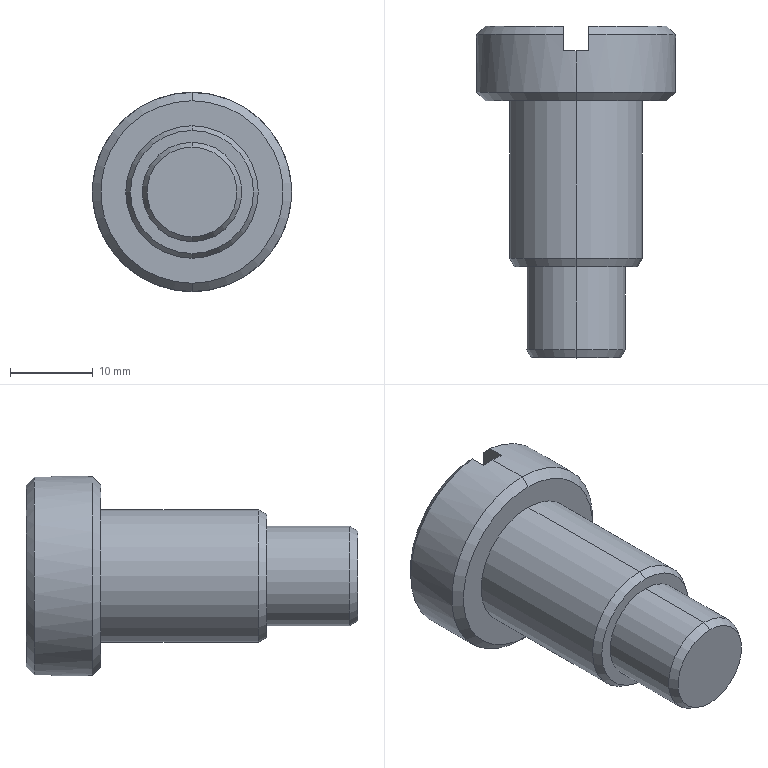Part | SolidWorks | features Chamfer 2, ICE 1, Revolution 1 | 1 solid | 22 faces | box 24 x 40 x 24 mm | volume 9026 mm3 | cone 8 | plane 8 | cylinder 6 | commonest cylinder face diameters 12 x2 16 x2 24 x2
STEP:
#1=CARTESIAN_POINT('',(0.,0.,-5.423));
#2=VERTEX_POINT('',#1);
#3=CARTESIAN_POINT('',(0.,0.,5.423));
#4=VERTEX_POINT('',#3);
#5=CARTESIAN_POINT('',(0.,0.,0.));
#6=DIRECTION('',(0.,-1.,0.));
#7=DIRECTION('',(0.,0.,-1.));
#8=AXIS2_PLACEMENT_3D('',#5,#6,#7);
#9=CIRCLE('',#8,5.423);
#10=EDGE_CURVE('',#2,#4,#9,.T.);
#11=ORIENTED_EDGE('',*,*,#10,.F.);
#12=CARTESIAN_POINT('',(0.,1.,-6.));
#13=VERTEX_POINT('',#12);
#14=CARTESIAN_POINT('',(0.,0.,-5.423));
#15=DIRECTION('',(0.,0.866,-0.5));
#16=VECTOR('',#15,1000.);
#17=LINE('',#14,#16);
#18=EDGE_CURVE('',#2,#13,#17,.T.);
#19=ORIENTED_EDGE('',*,*,#18,.T.);
#20=CARTESIAN_POINT('',(0.,1.,6.));
#21=VERTEX_POINT('',#20);
#22=CARTESIAN_POINT('',(0.,1.,0.));
#23=DIRECTION('',(0.,1.,0.));
#24=DIRECTION('',(0.,0.,-1.));
#25=AXIS2_PLACEMENT_3D('',#22,#23,#24);
#26=CIRCLE('',#25,6.);
#27=EDGE_CURVE('',#21,#13,#26,.T.);
#28=ORIENTED_EDGE('',*,*,#27,.F.);
#29=CARTESIAN_POINT('',(0.,0.,5.423));
#30=DIRECTION('',(0.,0.866,0.5));
#31=VECTOR('',#30,1000.);
#32=LINE('',#29,#31);
#33=EDGE_CURVE('',#4,#21,#32,.T.);
#34=ORIENTED_EDGE('',*,*,#33,.F.);
#35=EDGE_LOOP('',(#11,#19,#28,#34));
#36=FACE_OUTER_BOUND('',#35,.T.);
#37=CARTESIAN_POINT('',(0.,0.,0.));
#38=DIRECTION('',(0.,1.,0.));
#39=DIRECTION('',(0.,0.,1.));
#40=AXIS2_PLACEMENT_3D('',#37,#38,#39);
#41=CONICAL_SURFACE('',#40,5.423,0.5236);
#42=ADVANCED_FACE('',(#36),#41,.T.);
#43=CARTESIAN_POINT('',(0.,11.,-7.423));
#44=VERTEX_POINT('',#43);
#45=CARTESIAN_POINT('',(0.,11.,7.423));
#46=VERTEX_POINT('',#45);
#47=CARTESIAN_POINT('',(0.,11.,0.));
#48=DIRECTION('',(0.,-1.,0.));
#49=DIRECTION('',(0.,0.,-1.));
#50=AXIS2_PLACEMENT_3D('',#47,#48,#49);
#51=CIRCLE('',#50,7.423);
#52=EDGE_CURVE('',#44,#46,#51,.T.);
#53=ORIENTED_EDGE('',*,*,#52,.F.);
#54=CARTESIAN_POINT('',(0.,12.,-8.));
#55=VERTEX_POINT('',#54);
#56=CARTESIAN_POINT('',(0.,11.,-7.423));
#57=DIRECTION('',(0.,0.866,-0.5));
#58=VECTOR('',#57,1000.);
#59=LINE('',#56,#58);
#60=EDGE_CURVE('',#44,#55,#59,.T.);
#61=ORIENTED_EDGE('',*,*,#60,.T.);
#62=CARTESIAN_POINT('',(0.,12.,8.));
#63=VERTEX_POINT('',#62);
#64=CARTESIAN_POINT('',(0.,12.,0.));
#65=DIRECTION('',(0.,1.,0.));
#66=DIRECTION('',(0.,0.,-1.));
#67=AXIS2_PLACEMENT_3D('',#64,#65,#66);
#68=CIRCLE('',#67,8.);
#69=EDGE_CURVE('',#63,#55,#68,.T.);
#70=ORIENTED_EDGE('',*,*,#69,.F.);
#71=CARTESIAN_POINT('',(0.,11.,7.423));
#72=DIRECTION('',(0.,0.866,0.5));
#73=VECTOR('',#72,1000.);
#74=LINE('',#71,#73);
#75=EDGE_CURVE('',#46,#63,#74,.T.);
#76=ORIENTED_EDGE('',*,*,#75,.F.);
#77=EDGE_LOOP('',(#53,#61,#70,#76));
#78=FACE_OUTER_BOUND('',#77,.T.);
#79=CARTESIAN_POINT('',(0.,11.,0.));
#80=DIRECTION('',(0.,1.,0.));
#81=DIRECTION('',(0.,0.,1.));
#82=AXIS2_PLACEMENT_3D('',#79,#80,#81);
#83=CONICAL_SURFACE('',#82,7.423,0.5236);
#84=ADVANCED_FACE('',(#78),#83,.T.);
#85=CARTESIAN_POINT('',(0.,31.,-11.));
#86=VERTEX_POINT('',#85);
#87=CARTESIAN_POINT('',(0.,31.,11.));
#88=VERTEX_POINT('',#87);
#89=CARTESIAN_POINT('',(0.,31.,0.));
#90=DIRECTION('',(0.,-1.,0.));
#91=DIRECTION('',(0.,0.,-1.));
#92=AXIS2_PLACEMENT_3D('',#89,#90,#91);
#93=CIRCLE('',#92,11.);
#94=EDGE_CURVE('',#86,#88,#93,.T.);
#95=ORIENTED_EDGE('',*,*,#94,.F.);
#96=CARTESIAN_POINT('',(0.,32.,-12.));
#97=VERTEX_POINT('',#96);
#98=CARTESIAN_POINT('',(0.,31.,-11.));
#99=DIRECTION('',(0.,0.7071,-0.7071));
#100=VECTOR('',#99,1000.);
#101=LINE('',#98,#100);
#102=EDGE_CURVE('',#86,#97,#101,.T.);
#103=ORIENTED_EDGE('',*,*,#102,.T.);
#104=CARTESIAN_POINT('',(0.,32.,12.));
#105=VERTEX_POINT('',#104);
#106=CARTESIAN_POINT('',(0.,32.,0.));
#107=DIRECTION('',(0.,1.,0.));
#108=DIRECTION('',(0.,0.,-1.));
#109=AXIS2_PLACEMENT_3D('',#106,#107,#108);
#110=CIRCLE('',#109,12.);
#111=EDGE_CURVE('',#105,#97,#110,.T.);
#112=ORIENTED_EDGE('',*,*,#111,.F.);
#113=CARTESIAN_POINT('',(0.,31.,11.));
#114=DIRECTION('',(0.,0.7071,0.7071));
#115=VECTOR('',#114,1000.);
#116=LINE('',#113,#115);
#117=EDGE_CURVE('',#88,#105,#116,.T.);
#118=ORIENTED_EDGE('',*,*,#117,.F.);
#119=EDGE_LOOP('',(#95,#103,#112,#118));
#120=FACE_OUTER_BOUND('',#119,.T.);
#121=CARTESIAN_POINT('',(0.,31.,0.));
#122=DIRECTION('',(0.,1.,0.));
#123=DIRECTION('',(0.,0.,1.));
#124=AXIS2_PLACEMENT_3D('',#121,#122,#123);
#125=CONICAL_SURFACE('',#124,11.,0.7854);
#126=ADVANCED_FACE('',(#120),#125,.T.);
#127=CARTESIAN_POINT('',(0.,11.,-6.));
#128=VERTEX_POINT('',#127);
#129=CARTESIAN_POINT('',(0.,11.,6.));
#130=VERTEX_POINT('',#129);
#131=CARTESIAN_POINT('',(0.,11.,0.));
#132=DIRECTION('',(0.,-1.,0.));
#133=DIRECTION('',(0.,0.,-1.));
#134=AXIS2_PLACEMENT_3D('',#131,#132,#133);
#135=CIRCLE('',#134,6.);
#136=EDGE_CURVE('',#128,#130,#135,.T.);
#137=ORIENTED_EDGE('',*,*,#136,.T.);
#138=CARTESIAN_POINT('',(0.,0.,6.));
#139=DIRECTION('',(0.,-1.,0.));
#140=VECTOR('',#139,1000.);
#141=LINE('',#138,#140);
#142=EDGE_CURVE('',#130,#21,#141,.T.);
#143=ORIENTED_EDGE('',*,*,#142,.T.);
#144=ORIENTED_EDGE('',*,*,#27,.T.);
#145=CARTESIAN_POINT('',(0.,0.,-6.));
#146=DIRECTION('',(0.,-1.,0.));
#147=VECTOR('',#146,1000.);
#148=LINE('',#145,#147);
#149=EDGE_CURVE('',#128,#13,#148,.T.);
#150=ORIENTED_EDGE('',*,*,#149,.F.);
#151=EDGE_LOOP('',(#137,#143,#144,#150));
#152=FACE_OUTER_BOUND('',#151,.T.);
#153=CARTESIAN_POINT('',(0.,0.,0.));
#154=DIRECTION('',(0.,-1.,0.));
#155=DIRECTION('',(0.,0.,-1.));
#156=AXIS2_PLACEMENT_3D('',#153,#154,#155);
#157=CYLINDRICAL_SURFACE('',#156,6.);
#158=ADVANCED_FACE('',(#152),#157,.T.);
#159=CARTESIAN_POINT('',(0.,31.,-8.));
#160=VERTEX_POINT('',#159);
#161=CARTESIAN_POINT('',(0.,31.,8.));
#162=VERTEX_POINT('',#161);
#163=CARTESIAN_POINT('',(0.,31.,0.));
#164=DIRECTION('',(0.,-1.,0.));
#165=DIRECTION('',(0.,0.,-1.));
#166=AXIS2_PLACEMENT_3D('',#163,#164,#165);
#167=CIRCLE('',#166,8.);
#168=EDGE_CURVE('',#160,#162,#167,.T.);
#169=ORIENTED_EDGE('',*,*,#168,.T.);
#170=CARTESIAN_POINT('',(0.,0.,8.));
#171=DIRECTION('',(0.,-1.,0.));
#172=VECTOR('',#171,1000.);
#173=LINE('',#170,#172);
#174=EDGE_CURVE('',#162,#63,#173,.T.);
#175=ORIENTED_EDGE('',*,*,#174,.T.);
#176=ORIENTED_EDGE('',*,*,#69,.T.);
#177=CARTESIAN_POINT('',(0.,0.,-8.));
#178=DIRECTION('',(0.,-1.,0.));
#179=VECTOR('',#178,1000.);
#180=LINE('',#177,#179);
#181=EDGE_CURVE('',#160,#55,#180,.T.);
#182=ORIENTED_EDGE('',*,*,#181,.F.);
#183=EDGE_LOOP('',(#169,#175,#176,#182));
#184=FACE_OUTER_BOUND('',#183,.T.);
#185=CARTESIAN_POINT('',(0.,0.,0.));
#186=DIRECTION('',(0.,-1.,0.));
#187=DIRECTION('',(0.,0.,-1.));
#188=AXIS2_PLACEMENT_3D('',#185,#186,#187);
#189=CYLINDRICAL_SURFACE('',#188,8.);
#190=ADVANCED_FACE('',(#184),#189,.T.);
#191=CARTESIAN_POINT('',(0.,37.,12.));
#192=VERTEX_POINT('',#191);
#193=CARTESIAN_POINT('',(1.5,37.,11.906));
#194=VERTEX_POINT('',#193);
#195=CARTESIAN_POINT('',(0.,37.,0.));
#196=DIRECTION('',(0.,1.,0.));
#197=DIRECTION('',(0.,0.,-1.));
#198=AXIS2_PLACEMENT_3D('',#195,#196,#197);
#199=CIRCLE('',#198,12.);
#200=EDGE_CURVE('',#192,#194,#199,.T.);
#201=ORIENTED_EDGE('',*,*,#200,.F.);
#202=CARTESIAN_POINT('',(0.,0.,12.));
#203=DIRECTION('',(0.,-1.,0.));
#204=VECTOR('',#203,1000.);
#205=LINE('',#202,#204);
#206=EDGE_CURVE('',#192,#105,#205,.T.);
#207=ORIENTED_EDGE('',*,*,#206,.T.);
#208=ORIENTED_EDGE('',*,*,#111,.T.);
#209=CARTESIAN_POINT('',(0.,37.,-12.));
#210=VERTEX_POINT('',#209);
#211=CARTESIAN_POINT('',(0.,0.,-12.));
#212=DIRECTION('',(0.,-1.,0.));
#213=VECTOR('',#212,1000.);
#214=LINE('',#211,#213);
#215=EDGE_CURVE('',#210,#97,#214,.T.);
#216=ORIENTED_EDGE('',*,*,#215,.F.);
#217=CARTESIAN_POINT('',(1.5,37.,-11.906));
#218=VERTEX_POINT('',#217);
#219=CARTESIAN_POINT('',(0.,37.,0.));
#220=DIRECTION('',(0.,1.,0.));
#221=DIRECTION('',(0.,0.,-1.));
#222=AXIS2_PLACEMENT_3D('',#219,#220,#221);
#223=CIRCLE('',#222,12.);
#224=EDGE_CURVE('',#218,#210,#223,.T.);
#225=ORIENTED_EDGE('',*,*,#224,.F.);
#226=CARTESIAN_POINT('',(1.5,39.,-11.906));
#227=VERTEX_POINT('',#226);
#228=CARTESIAN_POINT('',(1.5,0.,-11.906));
#229=DIRECTION('',(0.,-1.,0.));
#230=VECTOR('',#229,1000.);
#231=LINE('',#228,#230);
#232=EDGE_CURVE('',#227,#218,#231,.T.);
#233=ORIENTED_EDGE('',*,*,#232,.F.);
#234=CARTESIAN_POINT('',(1.5,39.,11.906));
#235=VERTEX_POINT('',#234);
#236=CARTESIAN_POINT('',(0.,39.,0.));
#237=DIRECTION('',(0.,-1.,0.));
#238=DIRECTION('',(0.,0.,1.));
#239=AXIS2_PLACEMENT_3D('',#236,#237,#238);
#240=CIRCLE('',#239,12.);
#241=EDGE_CURVE('',#227,#235,#240,.T.);
#242=ORIENTED_EDGE('',*,*,#241,.T.);
#243=CARTESIAN_POINT('',(1.5,0.,11.906));
#244=DIRECTION('',(0.,1.,0.));
#245=VECTOR('',#244,1000.);
#246=LINE('',#243,#245);
#247=EDGE_CURVE('',#194,#235,#246,.T.);
#248=ORIENTED_EDGE('',*,*,#247,.F.);
#249=EDGE_LOOP('',(#201,#207,#208,#216,#225,#233,#242,#248));
#250=FACE_OUTER_BOUND('',#249,.T.);
#251=CARTESIAN_POINT('',(0.,0.,0.));
#252=DIRECTION('',(0.,-1.,0.));
#253=DIRECTION('',(0.,0.,-1.));
#254=AXIS2_PLACEMENT_3D('',#251,#252,#253);
#255=CYLINDRICAL_SURFACE('',#254,12.);
#256=ADVANCED_FACE('',(#250),#255,.T.);
#257=CARTESIAN_POINT('',(1.5,40.,10.897));
#258=VERTEX_POINT('',#257);
#259=CARTESIAN_POINT('',(1.5,40.,-10.897));
#260=VERTEX_POINT('',#259);
#261=CARTESIAN_POINT('',(1.5,40.,15.294));
#262=DIRECTION('',(0.,0.,-1.));
#263=VECTOR('',#262,1000.);
#264=LINE('',#261,#263);
#265=EDGE_CURVE('',#258,#260,#264,.T.);
#266=ORIENTED_EDGE('',*,*,#265,.F.);
#267=CARTESIAN_POINT('',(0.,40.,0.));
#268=DIRECTION('',(0.,1.,0.));
#269=DIRECTION('',(0.,0.,1.));
#270=AXIS2_PLACEMENT_3D('',#267,#268,#269);
#271=CIRCLE('',#270,11.);
#272=EDGE_CURVE('',#258,#260,#271,.T.);
#273=ORIENTED_EDGE('',*,*,#272,.T.);
#274=EDGE_LOOP('',(#266,#273));
#275=FACE_OUTER_BOUND('',#274,.T.);
#276=CARTESIAN_POINT('',(0.,40.,0.));
#277=DIRECTION('',(0.,1.,0.));
#278=DIRECTION('',(0.,0.,1.));
#279=AXIS2_PLACEMENT_3D('',#276,#277,#278);
#280=PLANE('',#279);
#281=ADVANCED_FACE('',(#275),#280,.T.);
#282=CARTESIAN_POINT('',(1.5,39.,11.906));
#283=CARTESIAN_POINT('',(1.5,39.333,11.57));
#284=CARTESIAN_POINT('',(1.5,39.667,11.234));
#285=CARTESIAN_POINT('',(1.5,40.,10.897));
#286=B_SPLINE_CURVE_WITH_KNOTS('',3,(#282,#283,#284,#285),.UNSPECIFIED.,.F.,.F.,(4,4),(0.000000994,0.001421),.UNSPECIFIED.);
#287=EDGE_CURVE('',#235,#258,#286,.T.);
#288=ORIENTED_EDGE('',*,*,#287,.F.);
#289=ORIENTED_EDGE('',*,*,#241,.F.);
#290=CARTESIAN_POINT('',(1.5,40.,-10.897));
#291=CARTESIAN_POINT('',(1.5,39.667,-11.234));
#292=CARTESIAN_POINT('',(1.5,39.333,-11.57));
#293=CARTESIAN_POINT('',(1.5,39.,-11.906));
#294=B_SPLINE_CURVE_WITH_KNOTS('',3,(#290,#291,#292,#293),.UNSPECIFIED.,.F.,.F.,(4,4),(0.03055,0.03197),.UNSPECIFIED.);
#295=EDGE_CURVE('',#260,#227,#294,.T.);
#296=ORIENTED_EDGE('',*,*,#295,.F.);
#297=ORIENTED_EDGE('',*,*,#272,.F.);
#298=EDGE_LOOP('',(#288,#289,#296,#297));
#299=FACE_OUTER_BOUND('',#298,.T.);
#300=CARTESIAN_POINT('',(0.,39.,0.));
#301=DIRECTION('',(0.,-1.,0.));
#302=DIRECTION('',(0.,0.,-1.));
#303=AXIS2_PLACEMENT_3D('',#300,#301,#302);
#304=CONICAL_SURFACE('',#303,12.,0.7854);
#305=ADVANCED_FACE('',(#299),#304,.T.);
#306=CARTESIAN_POINT('',(0.,0.,0.));
#307=DIRECTION('',(0.,-1.,0.));
#308=DIRECTION('',(0.,0.,-1.));
#309=AXIS2_PLACEMENT_3D('',#306,#307,#308);
#310=CIRCLE('',#309,5.423);
#311=EDGE_CURVE('',#4,#2,#310,.T.);
#312=ORIENTED_EDGE('',*,*,#311,.T.);
#313=ORIENTED_EDGE('',*,*,#10,.T.);
#314=EDGE_LOOP('',(#312,#313));
#315=FACE_OUTER_BOUND('',#314,.T.);
#316=CARTESIAN_POINT('',(6.,0.,0.));
#317=DIRECTION('',(0.,-1.,0.));
#318=DIRECTION('',(0.,0.,-1.));
#319=AXIS2_PLACEMENT_3D('',#316,#317,#318);
#320=PLANE('',#319);
#321=ADVANCED_FACE('',(#315),#320,.T.);
#322=CARTESIAN_POINT('',(-1.5,40.,-10.897));
#323=VERTEX_POINT('',#322);
#324=CARTESIAN_POINT('',(-1.5,40.,10.897));
#325=VERTEX_POINT('',#324);
#326=CARTESIAN_POINT('',(-1.5,40.,15.294));
#327=DIRECTION('',(0.,0.,1.));
#328=VECTOR('',#327,1000.);
#329=LINE('',#326,#328);
#330=EDGE_CURVE('',#323,#325,#329,.T.);
#331=ORIENTED_EDGE('',*,*,#330,.F.);
#332=CARTESIAN_POINT('',(0.,40.,0.));
#333=DIRECTION('',(0.,1.,0.));
#334=DIRECTION('',(0.,0.,1.));
#335=AXIS2_PLACEMENT_3D('',#332,#333,#334);
#336=CIRCLE('',#335,11.);
#337=EDGE_CURVE('',#323,#325,#336,.T.);
#338=ORIENTED_EDGE('',*,*,#337,.T.);
#339=EDGE_LOOP('',(#331,#338));
#340=FACE_OUTER_BOUND('',#339,.T.);
#341=CARTESIAN_POINT('',(0.,40.,0.));
#342=DIRECTION('',(0.,1.,0.));
#343=DIRECTION('',(0.,0.,1.));
#344=AXIS2_PLACEMENT_3D('',#341,#342,#343);
#345=PLANE('',#344);
#346=ADVANCED_FACE('',(#340),#345,.T.);
#347=ORIENTED_EDGE('',*,*,#206,.F.);
#348=CARTESIAN_POINT('',(-1.5,37.,11.906));
#349=VERTEX_POINT('',#348);
#350=CARTESIAN_POINT('',(0.,37.,0.));
#351=DIRECTION('',(0.,1.,0.));
#352=DIRECTION('',(0.,0.,-1.));
#353=AXIS2_PLACEMENT_3D('',#350,#351,#352);
#354=CIRCLE('',#353,12.);
#355=EDGE_CURVE('',#349,#192,#354,.T.);
#356=ORIENTED_EDGE('',*,*,#355,.F.);
#357=CARTESIAN_POINT('',(-1.5,39.,11.906));
#358=VERTEX_POINT('',#357);
#359=CARTESIAN_POINT('',(-1.5,0.,11.906));
#360=DIRECTION('',(0.,-1.,0.));
#361=VECTOR('',#360,1000.);
#362=LINE('',#359,#361);
#363=EDGE_CURVE('',#358,#349,#362,.T.);
#364=ORIENTED_EDGE('',*,*,#363,.F.);
#365=CARTESIAN_POINT('',(-1.5,39.,-11.906));
#366=VERTEX_POINT('',#365);
#367=CARTESIAN_POINT('',(0.,39.,0.));
#368=DIRECTION('',(0.,-1.,0.));
#369=DIRECTION('',(0.,0.,1.));
#370=AXIS2_PLACEMENT_3D('',#367,#368,#369);
#371=CIRCLE('',#370,12.);
#372=EDGE_CURVE('',#358,#366,#371,.T.);
#373=ORIENTED_EDGE('',*,*,#372,.T.);
#374=CARTESIAN_POINT('',(-1.5,37.,-11.906));
#375=VERTEX_POINT('',#374);
#376=CARTESIAN_POINT('',(-1.5,0.,-11.906));
#377=DIRECTION('',(0.,1.,0.));
#378=VECTOR('',#377,1000.);
#379=LINE('',#376,#378);
#380=EDGE_CURVE('',#375,#366,#379,.T.);
#381=ORIENTED_EDGE('',*,*,#380,.F.);
#382=CARTESIAN_POINT('',(0.,37.,0.));
#383=DIRECTION('',(0.,1.,0.));
#384=DIRECTION('',(0.,0.,-1.));
#385=AXIS2_PLACEMENT_3D('',#382,#383,#384);
#386=CIRCLE('',#385,12.);
#387=EDGE_CURVE('',#210,#375,#386,.T.);
#388=ORIENTED_EDGE('',*,*,#387,.F.);
#389=ORIENTED_EDGE('',*,*,#215,.T.);
#390=CARTESIAN_POINT('',(0.,32.,0.));
#391=DIRECTION('',(0.,1.,0.));
#392=DIRECTION('',(0.,0.,-1.));
#393=AXIS2_PLACEMENT_3D('',#390,#391,#392);
#394=CIRCLE('',#393,12.);
#395=EDGE_CURVE('',#97,#105,#394,.T.);
#396=ORIENTED_EDGE('',*,*,#395,.T.);
#397=EDGE_LOOP('',(#347,#356,#364,#373,#381,#388,#389,#396));
#398=FACE_OUTER_BOUND('',#397,.T.);
#399=CARTESIAN_POINT('',(0.,0.,0.));
#400=DIRECTION('',(0.,-1.,0.));
#401=DIRECTION('',(0.,0.,-1.));
#402=AXIS2_PLACEMENT_3D('',#399,#400,#401);
#403=CYLINDRICAL_SURFACE('',#402,12.);
#404=ADVANCED_FACE('',(#398),#403,.T.);
#405=CARTESIAN_POINT('',(0.,31.,0.));
#406=DIRECTION('',(0.,-1.,0.));
#407=DIRECTION('',(0.,0.,-1.));
#408=AXIS2_PLACEMENT_3D('',#405,#406,#407);
#409=CIRCLE('',#408,11.);
#410=EDGE_CURVE('',#88,#86,#409,.T.);
#411=ORIENTED_EDGE('',*,*,#410,.T.);
#412=ORIENTED_EDGE('',*,*,#94,.T.);
#413=EDGE_LOOP('',(#411,#412));
#414=FACE_OUTER_BOUND('',#413,.T.);
#415=ORIENTED_EDGE('',*,*,#168,.F.);
#416=CARTESIAN_POINT('',(0.,31.,0.));
#417=DIRECTION('',(0.,-1.,0.));
#418=DIRECTION('',(0.,0.,-1.));
#419=AXIS2_PLACEMENT_3D('',#416,#417,#418);
#420=CIRCLE('',#419,8.);
#421=EDGE_CURVE('',#162,#160,#420,.T.);
#422=ORIENTED_EDGE('',*,*,#421,.F.);
#423=EDGE_LOOP('',(#415,#422));
#424=FACE_BOUND('',#423,.T.);
#425=CARTESIAN_POINT('',(12.,31.,0.));
#426=DIRECTION('',(0.,-1.,0.));
#427=DIRECTION('',(0.,0.,-1.));
#428=AXIS2_PLACEMENT_3D('',#425,#426,#427);
#429=PLANE('',#428);
#430=ADVANCED_FACE('',(#414,#424),#429,.T.);
#431=ORIENTED_EDGE('',*,*,#174,.F.);
#432=ORIENTED_EDGE('',*,*,#421,.T.);
#433=ORIENTED_EDGE('',*,*,#181,.T.);
#434=CARTESIAN_POINT('',(0.,12.,0.));
#435=DIRECTION('',(0.,1.,0.));
#436=DIRECTION('',(0.,0.,-1.));
#437=AXIS2_PLACEMENT_3D('',#434,#435,#436);
#438=CIRCLE('',#437,8.);
#439=EDGE_CURVE('',#55,#63,#438,.T.);
#440=ORIENTED_EDGE('',*,*,#439,.T.);
#441=EDGE_LOOP('',(#431,#432,#433,#440));
#442=FACE_OUTER_BOUND('',#441,.T.);
#443=CARTESIAN_POINT('',(0.,0.,0.));
#444=DIRECTION('',(0.,-1.,0.));
#445=DIRECTION('',(0.,0.,-1.));
#446=AXIS2_PLACEMENT_3D('',#443,#444,#445);
#447=CYLINDRICAL_SURFACE('',#446,8.);
#448=ADVANCED_FACE('',(#442),#447,.T.);
#449=CARTESIAN_POINT('',(0.,11.,0.));
#450=DIRECTION('',(0.,-1.,0.));
#451=DIRECTION('',(0.,0.,-1.));
#452=AXIS2_PLACEMENT_3D('',#449,#450,#451);
#453=CIRCLE('',#452,7.423);
#454=EDGE_CURVE('',#46,#44,#453,.T.);
#455=ORIENTED_EDGE('',*,*,#454,.T.);
#456=ORIENTED_EDGE('',*,*,#52,.T.);
#457=EDGE_LOOP('',(#455,#456));
#458=FACE_OUTER_BOUND('',#457,.T.);
#459=ORIENTED_EDGE('',*,*,#136,.F.);
#460=CARTESIAN_POINT('',(0.,11.,0.));
#461=DIRECTION('',(0.,-1.,0.));
#462=DIRECTION('',(0.,0.,-1.));
#463=AXIS2_PLACEMENT_3D('',#460,#461,#462);
#464=CIRCLE('',#463,6.);
#465=EDGE_CURVE('',#130,#128,#464,.T.);
#466=ORIENTED_EDGE('',*,*,#465,.F.);
#467=EDGE_LOOP('',(#459,#466));
#468=FACE_BOUND('',#467,.T.);
#469=CARTESIAN_POINT('',(8.,11.,0.));
#470=DIRECTION('',(0.,-1.,0.));
#471=DIRECTION('',(0.,0.,-1.));
#472=AXIS2_PLACEMENT_3D('',#469,#470,#471);
#473=PLANE('',#472);
#474=ADVANCED_FACE('',(#458,#468),#473,.T.);
#475=ORIENTED_EDGE('',*,*,#142,.F.);
#476=ORIENTED_EDGE('',*,*,#465,.T.);
#477=ORIENTED_EDGE('',*,*,#149,.T.);
#478=CARTESIAN_POINT('',(0.,1.,0.));
#479=DIRECTION('',(0.,1.,0.));
#480=DIRECTION('',(0.,0.,-1.));
#481=AXIS2_PLACEMENT_3D('',#478,#479,#480);
#482=CIRCLE('',#481,6.);
#483=EDGE_CURVE('',#13,#21,#482,.T.);
#484=ORIENTED_EDGE('',*,*,#483,.T.);
#485=EDGE_LOOP('',(#475,#476,#477,#484));
#486=FACE_OUTER_BOUND('',#485,.T.);
#487=CARTESIAN_POINT('',(0.,0.,0.));
#488=DIRECTION('',(0.,-1.,0.));
#489=DIRECTION('',(0.,0.,-1.));
#490=AXIS2_PLACEMENT_3D('',#487,#488,#489);
#491=CYLINDRICAL_SURFACE('',#490,6.);
#492=ADVANCED_FACE('',(#486),#491,.T.);
#493=CARTESIAN_POINT('',(-1.5,39.,-11.906));
#494=CARTESIAN_POINT('',(-1.5,39.333,-11.57));
#495=CARTESIAN_POINT('',(-1.5,39.667,-11.234));
#496=CARTESIAN_POINT('',(-1.5,40.,-10.897));
#497=B_SPLINE_CURVE_WITH_KNOTS('',3,(#493,#494,#495,#496),.UNSPECIFIED.,.F.,.F.,(4,4),(0.000000994,0.001421),.UNSPECIFIED.);
#498=EDGE_CURVE('',#366,#323,#497,.T.);
#499=ORIENTED_EDGE('',*,*,#498,.F.);
#500=ORIENTED_EDGE('',*,*,#372,.F.);
#501=CARTESIAN_POINT('',(-1.5,40.,10.897));
#502=CARTESIAN_POINT('',(-1.5,39.667,11.234));
#503=CARTESIAN_POINT('',(-1.5,39.333,11.57));
#504=CARTESIAN_POINT('',(-1.5,39.,11.906));
#505=B_SPLINE_CURVE_WITH_KNOTS('',3,(#501,#502,#503,#504),.UNSPECIFIED.,.F.,.F.,(4,4),(0.03055,0.03197),.UNSPECIFIED.);
#506=EDGE_CURVE('',#325,#358,#505,.T.);
#507=ORIENTED_EDGE('',*,*,#506,.F.);
#508=ORIENTED_EDGE('',*,*,#337,.F.);
#509=EDGE_LOOP('',(#499,#500,#507,#508));
#510=FACE_OUTER_BOUND('',#509,.T.);
#511=CARTESIAN_POINT('',(0.,39.,0.));
#512=DIRECTION('',(0.,-1.,0.));
#513=DIRECTION('',(0.,0.,-1.));
#514=AXIS2_PLACEMENT_3D('',#511,#512,#513);
#515=CONICAL_SURFACE('',#514,12.,0.7854);
#516=ADVANCED_FACE('',(#510),#515,.T.);
#517=ORIENTED_EDGE('',*,*,#102,.F.);
#518=ORIENTED_EDGE('',*,*,#410,.F.);
#519=ORIENTED_EDGE('',*,*,#117,.T.);
#520=ORIENTED_EDGE('',*,*,#395,.F.);
#521=EDGE_LOOP('',(#517,#518,#519,#520));
#522=FACE_OUTER_BOUND('',#521,.T.);
#523=CARTESIAN_POINT('',(0.,31.,0.));
#524=DIRECTION('',(0.,1.,0.));
#525=DIRECTION('',(0.,0.,1.));
#526=AXIS2_PLACEMENT_3D('',#523,#524,#525);
#527=CONICAL_SURFACE('',#526,11.,0.7854);
#528=ADVANCED_FACE('',(#522),#527,.T.);
#529=ORIENTED_EDGE('',*,*,#60,.F.);
#530=ORIENTED_EDGE('',*,*,#454,.F.);
#531=ORIENTED_EDGE('',*,*,#75,.T.);
#532=ORIENTED_EDGE('',*,*,#439,.F.);
#533=EDGE_LOOP('',(#529,#530,#531,#532));
#534=FACE_OUTER_BOUND('',#533,.T.);
#535=CARTESIAN_POINT('',(0.,11.,0.));
#536=DIRECTION('',(0.,1.,0.));
#537=DIRECTION('',(0.,0.,1.));
#538=AXIS2_PLACEMENT_3D('',#535,#536,#537);
#539=CONICAL_SURFACE('',#538,7.423,0.5236);
#540=ADVANCED_FACE('',(#534),#539,.T.);
#541=ORIENTED_EDGE('',*,*,#18,.F.);
#542=ORIENTED_EDGE('',*,*,#311,.F.);
#543=ORIENTED_EDGE('',*,*,#33,.T.);
#544=ORIENTED_EDGE('',*,*,#483,.F.);
#545=EDGE_LOOP('',(#541,#542,#543,#544));
#546=FACE_OUTER_BOUND('',#545,.T.);
#547=CARTESIAN_POINT('',(0.,0.,0.));
#548=DIRECTION('',(0.,1.,0.));
#549=DIRECTION('',(0.,0.,1.));
#550=AXIS2_PLACEMENT_3D('',#547,#548,#549);
#551=CONICAL_SURFACE('',#550,5.423,0.5236);
#552=ADVANCED_FACE('',(#546),#551,.T.);
#553=ORIENTED_EDGE('',*,*,#247,.T.);
#554=ORIENTED_EDGE('',*,*,#287,.T.);
#555=ORIENTED_EDGE('',*,*,#265,.T.);
#556=ORIENTED_EDGE('',*,*,#295,.T.);
#557=ORIENTED_EDGE('',*,*,#232,.T.);
#558=CARTESIAN_POINT('',(1.5,37.,15.294));
#559=DIRECTION('',(0.,0.,-1.));
#560=VECTOR('',#559,1000.);
#561=LINE('',#558,#560);
#562=EDGE_CURVE('',#194,#218,#561,.T.);
#563=ORIENTED_EDGE('',*,*,#562,.F.);
#564=EDGE_LOOP('',(#553,#554,#555,#556,#557,#563));
#565=FACE_OUTER_BOUND('',#564,.T.);
#566=CARTESIAN_POINT('',(1.5,37.,15.294));
#567=DIRECTION('',(1.,0.,0.));
#568=DIRECTION('',(0.,0.,-1.));
#569=AXIS2_PLACEMENT_3D('',#566,#567,#568);
#570=PLANE('',#569);
#571=ADVANCED_FACE('',(#565),#570,.F.);
#572=ORIENTED_EDGE('',*,*,#380,.T.);
#573=ORIENTED_EDGE('',*,*,#498,.T.);
#574=ORIENTED_EDGE('',*,*,#330,.T.);
#575=ORIENTED_EDGE('',*,*,#506,.T.);
#576=ORIENTED_EDGE('',*,*,#363,.T.);
#577=CARTESIAN_POINT('',(-1.5,37.,15.294));
#578=DIRECTION('',(0.,0.,1.));
#579=VECTOR('',#578,1000.);
#580=LINE('',#577,#579);
#581=EDGE_CURVE('',#375,#349,#580,.T.);
#582=ORIENTED_EDGE('',*,*,#581,.F.);
#583=EDGE_LOOP('',(#572,#573,#574,#575,#576,#582));
#584=FACE_OUTER_BOUND('',#583,.T.);
#585=CARTESIAN_POINT('',(-1.5,37.,15.294));
#586=DIRECTION('',(-1.,0.,0.));
#587=DIRECTION('',(0.,0.,1.));
#588=AXIS2_PLACEMENT_3D('',#585,#586,#587);
#589=PLANE('',#588);
#590=ADVANCED_FACE('',(#584),#589,.F.);
#591=ORIENTED_EDGE('',*,*,#355,.T.);
#592=ORIENTED_EDGE('',*,*,#200,.T.);
#593=ORIENTED_EDGE('',*,*,#562,.T.);
#594=ORIENTED_EDGE('',*,*,#224,.T.);
#595=ORIENTED_EDGE('',*,*,#387,.T.);
#596=ORIENTED_EDGE('',*,*,#581,.T.);
#597=EDGE_LOOP('',(#591,#592,#593,#594,#595,#596));
#598=FACE_OUTER_BOUND('',#597,.T.);
#599=CARTESIAN_POINT('',(0.,37.,0.));
#600=DIRECTION('',(0.,-1.,0.));
#601=DIRECTION('',(0.,0.,-1.));
#602=AXIS2_PLACEMENT_3D('',#599,#600,#601);
#603=PLANE('',#602);
#604=ADVANCED_FACE('',(#598),#603,.F.);
#605=CLOSED_SHELL('',(#42,#84,#126,#158,#190,#256,#281,#305,#321,#346,#404,#430,#448,#474,#492,#516,#528,#540,#552,#571,#590,#604));
#606=MANIFOLD_SOLID_BREP('',#605);
#607=CARTESIAN_POINT('',(0.,0.,0.));
#608=DIRECTION('',(0.,0.,1.));
#609=DIRECTION('',(1.,0.,0.));
#610=AXIS2_PLACEMENT_3D('',#607,#608,#609);
#611=(LENGTH_UNIT()NAMED_UNIT(*)SI_UNIT(.MILLI.,.METRE.));
#612=UNCERTAINTY_MEASURE_WITH_UNIT(LENGTH_MEASURE(0.00001),#611,'','');
#613=(NAMED_UNIT(*)PLANE_ANGLE_UNIT()SI_UNIT($,.RADIAN.));
#614=(NAMED_UNIT(*)SI_UNIT($,.STERADIAN.)SOLID_ANGLE_UNIT());
#615=(GEOMETRIC_REPRESENTATION_CONTEXT(3)GLOBAL_UNCERTAINTY_ASSIGNED_CONTEXT((#612))GLOBAL_UNIT_ASSIGNED_CONTEXT((#611,#613,#614))REPRESENTATION_CONTEXT('',''));
#616=ADVANCED_BREP_SHAPE_REPRESENTATION('',(#606,#610),#615);